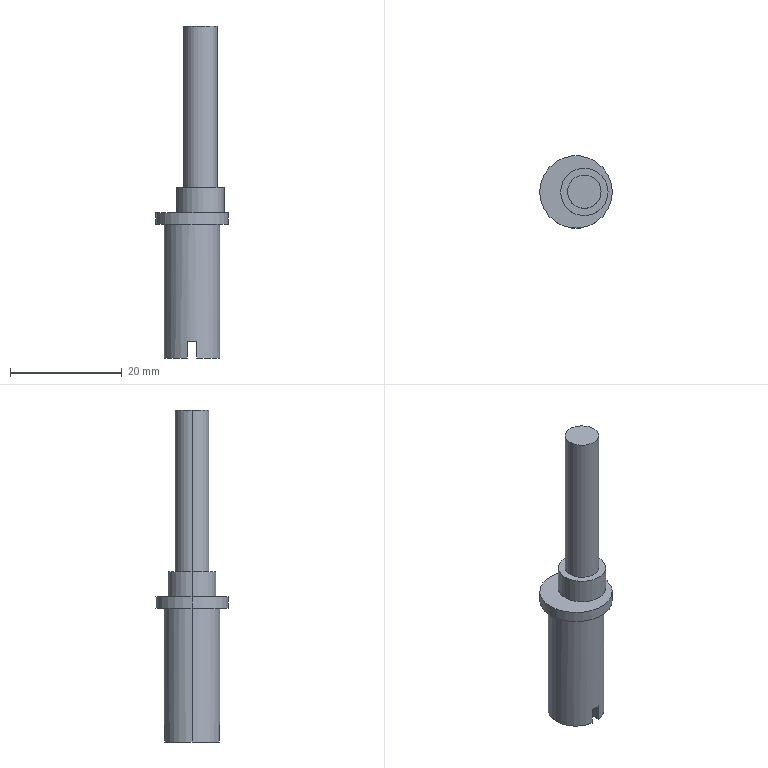Part | SolidWorks | features ICE 5, Extrusion 1 | 1 solid | 17 faces | box 13 x 13 x 59.5 mm | volume 3175 mm3 | plane 9 | cylinder 8 | commonest cylinder face diameters 6 x2 8.5 x2 10 x2 13 x2
STEP:
#1=CARTESIAN_POINT('',(-5.,0.,24.));
#2=VERTEX_POINT('',#1);
#3=CARTESIAN_POINT('',(5.,0.,24.));
#4=VERTEX_POINT('',#3);
#5=CARTESIAN_POINT('',(0.,0.,24.));
#6=DIRECTION('',(0.,0.,-1.));
#7=DIRECTION('',(-1.,0.,0.));
#8=AXIS2_PLACEMENT_3D('',#5,#6,#7);
#9=CIRCLE('',#8,5.);
#10=EDGE_CURVE('',#2,#4,#9,.T.);
#11=ORIENTED_EDGE('',*,*,#10,.T.);
#12=CARTESIAN_POINT('',(5.,0.,0.));
#13=VERTEX_POINT('',#12);
#14=CARTESIAN_POINT('',(5.,0.,25.));
#15=DIRECTION('',(0.,0.,-1.));
#16=VECTOR('',#15,1000.);
#17=LINE('',#14,#16);
#18=EDGE_CURVE('',#4,#13,#17,.T.);
#19=ORIENTED_EDGE('',*,*,#18,.T.);
#20=CARTESIAN_POINT('',(0.85,4.927,0.));
#21=VERTEX_POINT('',#20);
#22=CARTESIAN_POINT('',(0.,0.,0.));
#23=DIRECTION('',(0.,0.,1.));
#24=DIRECTION('',(1.,0.,0.));
#25=AXIS2_PLACEMENT_3D('',#22,#23,#24);
#26=CIRCLE('',#25,5.);
#27=EDGE_CURVE('',#13,#21,#26,.T.);
#28=ORIENTED_EDGE('',*,*,#27,.T.);
#29=CARTESIAN_POINT('',(0.85,4.927,3.));
#30=VERTEX_POINT('',#29);
#31=CARTESIAN_POINT('',(0.85,4.927,25.));
#32=DIRECTION('',(0.,0.,1.));
#33=VECTOR('',#32,1000.);
#34=LINE('',#31,#33);
#35=EDGE_CURVE('',#21,#30,#34,.T.);
#36=ORIENTED_EDGE('',*,*,#35,.T.);
#37=CARTESIAN_POINT('',(-0.85,4.927,3.));
#38=VERTEX_POINT('',#37);
#39=CARTESIAN_POINT('',(0.,0.,3.));
#40=DIRECTION('',(0.,0.,-1.));
#41=DIRECTION('',(-1.,0.,0.));
#42=AXIS2_PLACEMENT_3D('',#39,#40,#41);
#43=CIRCLE('',#42,5.);
#44=EDGE_CURVE('',#38,#30,#43,.T.);
#45=ORIENTED_EDGE('',*,*,#44,.F.);
#46=CARTESIAN_POINT('',(-0.85,4.927,0.));
#47=VERTEX_POINT('',#46);
#48=CARTESIAN_POINT('',(-0.85,4.927,25.));
#49=DIRECTION('',(0.,0.,-1.));
#50=VECTOR('',#49,1000.);
#51=LINE('',#48,#50);
#52=EDGE_CURVE('',#38,#47,#51,.T.);
#53=ORIENTED_EDGE('',*,*,#52,.T.);
#54=CARTESIAN_POINT('',(-5.,0.,0.));
#55=VERTEX_POINT('',#54);
#56=CARTESIAN_POINT('',(0.,0.,0.));
#57=DIRECTION('',(0.,0.,1.));
#58=DIRECTION('',(1.,0.,0.));
#59=AXIS2_PLACEMENT_3D('',#56,#57,#58);
#60=CIRCLE('',#59,5.);
#61=EDGE_CURVE('',#47,#55,#60,.T.);
#62=ORIENTED_EDGE('',*,*,#61,.T.);
#63=CARTESIAN_POINT('',(-5.,0.,25.));
#64=DIRECTION('',(0.,0.,-1.));
#65=VECTOR('',#64,1000.);
#66=LINE('',#63,#65);
#67=EDGE_CURVE('',#2,#55,#66,.T.);
#68=ORIENTED_EDGE('',*,*,#67,.F.);
#69=EDGE_LOOP('',(#11,#19,#28,#36,#45,#53,#62,#68));
#70=FACE_OUTER_BOUND('',#69,.T.);
#71=CARTESIAN_POINT('',(0.,0.,25.));
#72=DIRECTION('',(0.,0.,-1.));
#73=DIRECTION('',(-1.,0.,0.));
#74=AXIS2_PLACEMENT_3D('',#71,#72,#73);
#75=CYLINDRICAL_SURFACE('',#74,5.);
#76=ADVANCED_FACE('',(#70),#75,.T.);
#77=CARTESIAN_POINT('',(4.5,0.,59.5));
#78=VERTEX_POINT('',#77);
#79=CARTESIAN_POINT('',(-1.5,0.,59.5));
#80=VERTEX_POINT('',#79);
#81=CARTESIAN_POINT('',(1.5,0.,59.5));
#82=DIRECTION('',(0.,0.,1.));
#83=DIRECTION('',(1.,0.,0.));
#84=AXIS2_PLACEMENT_3D('',#81,#82,#83);
#85=CIRCLE('',#84,3.);
#86=EDGE_CURVE('',#78,#80,#85,.T.);
#87=ORIENTED_EDGE('',*,*,#86,.F.);
#88=CARTESIAN_POINT('',(4.5,0.,30.5));
#89=VERTEX_POINT('',#88);
#90=CARTESIAN_POINT('',(4.5,0.,59.5));
#91=DIRECTION('',(0.,0.,-1.));
#92=VECTOR('',#91,1000.);
#93=LINE('',#90,#92);
#94=EDGE_CURVE('',#78,#89,#93,.T.);
#95=ORIENTED_EDGE('',*,*,#94,.T.);
#96=CARTESIAN_POINT('',(-1.5,0.,30.5));
#97=VERTEX_POINT('',#96);
#98=CARTESIAN_POINT('',(1.5,0.,30.5));
#99=DIRECTION('',(0.,0.,1.));
#100=DIRECTION('',(1.,0.,0.));
#101=AXIS2_PLACEMENT_3D('',#98,#99,#100);
#102=CIRCLE('',#101,3.);
#103=EDGE_CURVE('',#89,#97,#102,.T.);
#104=ORIENTED_EDGE('',*,*,#103,.T.);
#105=CARTESIAN_POINT('',(-1.5,0.,59.5));
#106=DIRECTION('',(0.,0.,-1.));
#107=VECTOR('',#106,1000.);
#108=LINE('',#105,#107);
#109=EDGE_CURVE('',#80,#97,#108,.T.);
#110=ORIENTED_EDGE('',*,*,#109,.F.);
#111=EDGE_LOOP('',(#87,#95,#104,#110));
#112=FACE_OUTER_BOUND('',#111,.T.);
#113=CARTESIAN_POINT('',(1.5,0.,59.5));
#114=DIRECTION('',(0.,0.,-1.));
#115=DIRECTION('',(-1.,0.,0.));
#116=AXIS2_PLACEMENT_3D('',#113,#114,#115);
#117=CYLINDRICAL_SURFACE('',#116,3.);
#118=ADVANCED_FACE('',(#112),#117,.T.);
#119=CARTESIAN_POINT('',(5.75,0.,30.5));
#120=VERTEX_POINT('',#119);
#121=CARTESIAN_POINT('',(-2.75,0.,30.5));
#122=VERTEX_POINT('',#121);
#123=CARTESIAN_POINT('',(1.5,0.,30.5));
#124=DIRECTION('',(0.,0.,1.));
#125=DIRECTION('',(1.,0.,0.));
#126=AXIS2_PLACEMENT_3D('',#123,#124,#125);
#127=CIRCLE('',#126,4.25);
#128=EDGE_CURVE('',#120,#122,#127,.T.);
#129=ORIENTED_EDGE('',*,*,#128,.F.);
#130=CARTESIAN_POINT('',(5.75,0.,26.));
#131=VERTEX_POINT('',#130);
#132=CARTESIAN_POINT('',(5.75,0.,30.5));
#133=DIRECTION('',(0.,0.,-1.));
#134=VECTOR('',#133,1000.);
#135=LINE('',#132,#134);
#136=EDGE_CURVE('',#120,#131,#135,.T.);
#137=ORIENTED_EDGE('',*,*,#136,.T.);
#138=CARTESIAN_POINT('',(-2.75,0.,26.));
#139=VERTEX_POINT('',#138);
#140=CARTESIAN_POINT('',(1.5,0.,26.));
#141=DIRECTION('',(0.,0.,1.));
#142=DIRECTION('',(1.,0.,0.));
#143=AXIS2_PLACEMENT_3D('',#140,#141,#142);
#144=CIRCLE('',#143,4.25);
#145=EDGE_CURVE('',#131,#139,#144,.T.);
#146=ORIENTED_EDGE('',*,*,#145,.T.);
#147=CARTESIAN_POINT('',(-2.75,0.,30.5));
#148=DIRECTION('',(0.,0.,-1.));
#149=VECTOR('',#148,1000.);
#150=LINE('',#147,#149);
#151=EDGE_CURVE('',#122,#139,#150,.T.);
#152=ORIENTED_EDGE('',*,*,#151,.F.);
#153=EDGE_LOOP('',(#129,#137,#146,#152));
#154=FACE_OUTER_BOUND('',#153,.T.);
#155=CARTESIAN_POINT('',(1.5,0.,30.5));
#156=DIRECTION('',(0.,0.,-1.));
#157=DIRECTION('',(-1.,0.,0.));
#158=AXIS2_PLACEMENT_3D('',#155,#156,#157);
#159=CYLINDRICAL_SURFACE('',#158,4.25);
#160=ADVANCED_FACE('',(#154),#159,.T.);
#161=CARTESIAN_POINT('',(6.5,0.,26.));
#162=VERTEX_POINT('',#161);
#163=CARTESIAN_POINT('',(-6.5,0.,26.));
#164=VERTEX_POINT('',#163);
#165=CARTESIAN_POINT('',(0.,0.,26.));
#166=DIRECTION('',(0.,0.,1.));
#167=DIRECTION('',(1.,0.,0.));
#168=AXIS2_PLACEMENT_3D('',#165,#166,#167);
#169=CIRCLE('',#168,6.5);
#170=EDGE_CURVE('',#162,#164,#169,.T.);
#171=ORIENTED_EDGE('',*,*,#170,.F.);
#172=CARTESIAN_POINT('',(6.5,0.,24.));
#173=VERTEX_POINT('',#172);
#174=CARTESIAN_POINT('',(6.5,0.,26.));
#175=DIRECTION('',(0.,0.,-1.));
#176=VECTOR('',#175,1000.);
#177=LINE('',#174,#176);
#178=EDGE_CURVE('',#162,#173,#177,.T.);
#179=ORIENTED_EDGE('',*,*,#178,.T.);
#180=CARTESIAN_POINT('',(-6.5,0.,24.));
#181=VERTEX_POINT('',#180);
#182=CARTESIAN_POINT('',(0.,0.,24.));
#183=DIRECTION('',(0.,0.,-1.));
#184=DIRECTION('',(-1.,0.,0.));
#185=AXIS2_PLACEMENT_3D('',#182,#183,#184);
#186=CIRCLE('',#185,6.5);
#187=EDGE_CURVE('',#181,#173,#186,.T.);
#188=ORIENTED_EDGE('',*,*,#187,.F.);
#189=CARTESIAN_POINT('',(-6.5,0.,26.));
#190=DIRECTION('',(0.,0.,-1.));
#191=VECTOR('',#190,1000.);
#192=LINE('',#189,#191);
#193=EDGE_CURVE('',#164,#181,#192,.T.);
#194=ORIENTED_EDGE('',*,*,#193,.F.);
#195=EDGE_LOOP('',(#171,#179,#188,#194));
#196=FACE_OUTER_BOUND('',#195,.T.);
#197=CARTESIAN_POINT('',(0.,0.,26.));
#198=DIRECTION('',(0.,0.,-1.));
#199=DIRECTION('',(-1.,0.,0.));
#200=AXIS2_PLACEMENT_3D('',#197,#198,#199);
#201=CYLINDRICAL_SURFACE('',#200,6.5);
#202=ADVANCED_FACE('',(#196),#201,.T.);
#203=ORIENTED_EDGE('',*,*,#178,.F.);
#204=CARTESIAN_POINT('',(0.,0.,26.));
#205=DIRECTION('',(0.,0.,1.));
#206=DIRECTION('',(1.,0.,0.));
#207=AXIS2_PLACEMENT_3D('',#204,#205,#206);
#208=CIRCLE('',#207,6.5);
#209=EDGE_CURVE('',#164,#162,#208,.T.);
#210=ORIENTED_EDGE('',*,*,#209,.F.);
#211=ORIENTED_EDGE('',*,*,#193,.T.);
#212=CARTESIAN_POINT('',(0.,0.,24.));
#213=DIRECTION('',(0.,0.,-1.));
#214=DIRECTION('',(-1.,0.,0.));
#215=AXIS2_PLACEMENT_3D('',#212,#213,#214);
#216=CIRCLE('',#215,6.5);
#217=EDGE_CURVE('',#173,#181,#216,.T.);
#218=ORIENTED_EDGE('',*,*,#217,.F.);
#219=EDGE_LOOP('',(#203,#210,#211,#218));
#220=FACE_OUTER_BOUND('',#219,.T.);
#221=CARTESIAN_POINT('',(0.,0.,26.));
#222=DIRECTION('',(0.,0.,-1.));
#223=DIRECTION('',(-1.,0.,0.));
#224=AXIS2_PLACEMENT_3D('',#221,#222,#223);
#225=CYLINDRICAL_SURFACE('',#224,6.5);
#226=ADVANCED_FACE('',(#220),#225,.T.);
#227=CARTESIAN_POINT('',(1.5,0.,26.));
#228=DIRECTION('',(0.,0.,1.));
#229=DIRECTION('',(1.,0.,0.));
#230=AXIS2_PLACEMENT_3D('',#227,#228,#229);
#231=CIRCLE('',#230,4.25);
#232=EDGE_CURVE('',#139,#131,#231,.T.);
#233=ORIENTED_EDGE('',*,*,#232,.F.);
#234=ORIENTED_EDGE('',*,*,#145,.F.);
#235=EDGE_LOOP('',(#233,#234));
#236=FACE_BOUND('',#235,.T.);
#237=ORIENTED_EDGE('',*,*,#209,.T.);
#238=ORIENTED_EDGE('',*,*,#170,.T.);
#239=EDGE_LOOP('',(#237,#238));
#240=FACE_OUTER_BOUND('',#239,.T.);
#241=CARTESIAN_POINT('',(0.,0.,26.));
#242=DIRECTION('',(0.,0.,1.));
#243=DIRECTION('',(1.,0.,0.));
#244=AXIS2_PLACEMENT_3D('',#241,#242,#243);
#245=PLANE('',#244);
#246=ADVANCED_FACE('',(#236,#240),#245,.T.);
#247=ORIENTED_EDGE('',*,*,#136,.F.);
#248=CARTESIAN_POINT('',(1.5,0.,30.5));
#249=DIRECTION('',(0.,0.,1.));
#250=DIRECTION('',(1.,0.,0.));
#251=AXIS2_PLACEMENT_3D('',#248,#249,#250);
#252=CIRCLE('',#251,4.25);
#253=EDGE_CURVE('',#122,#120,#252,.T.);
#254=ORIENTED_EDGE('',*,*,#253,.F.);
#255=ORIENTED_EDGE('',*,*,#151,.T.);
#256=ORIENTED_EDGE('',*,*,#232,.T.);
#257=EDGE_LOOP('',(#247,#254,#255,#256));
#258=FACE_OUTER_BOUND('',#257,.T.);
#259=CARTESIAN_POINT('',(1.5,0.,30.5));
#260=DIRECTION('',(0.,0.,-1.));
#261=DIRECTION('',(-1.,0.,0.));
#262=AXIS2_PLACEMENT_3D('',#259,#260,#261);
#263=CYLINDRICAL_SURFACE('',#262,4.25);
#264=ADVANCED_FACE('',(#258),#263,.T.);
#265=CARTESIAN_POINT('',(1.5,0.,30.5));
#266=DIRECTION('',(0.,0.,1.));
#267=DIRECTION('',(1.,0.,0.));
#268=AXIS2_PLACEMENT_3D('',#265,#266,#267);
#269=CIRCLE('',#268,3.);
#270=EDGE_CURVE('',#97,#89,#269,.T.);
#271=ORIENTED_EDGE('',*,*,#270,.F.);
#272=ORIENTED_EDGE('',*,*,#103,.F.);
#273=EDGE_LOOP('',(#271,#272));
#274=FACE_BOUND('',#273,.T.);
#275=ORIENTED_EDGE('',*,*,#253,.T.);
#276=ORIENTED_EDGE('',*,*,#128,.T.);
#277=EDGE_LOOP('',(#275,#276));
#278=FACE_OUTER_BOUND('',#277,.T.);
#279=CARTESIAN_POINT('',(1.5,0.,30.5));
#280=DIRECTION('',(0.,0.,1.));
#281=DIRECTION('',(1.,0.,0.));
#282=AXIS2_PLACEMENT_3D('',#279,#280,#281);
#283=PLANE('',#282);
#284=ADVANCED_FACE('',(#274,#278),#283,.T.);
#285=ORIENTED_EDGE('',*,*,#94,.F.);
#286=CARTESIAN_POINT('',(1.5,0.,59.5));
#287=DIRECTION('',(0.,0.,1.));
#288=DIRECTION('',(1.,0.,0.));
#289=AXIS2_PLACEMENT_3D('',#286,#287,#288);
#290=CIRCLE('',#289,3.);
#291=EDGE_CURVE('',#80,#78,#290,.T.);
#292=ORIENTED_EDGE('',*,*,#291,.F.);
#293=ORIENTED_EDGE('',*,*,#109,.T.);
#294=ORIENTED_EDGE('',*,*,#270,.T.);
#295=EDGE_LOOP('',(#285,#292,#293,#294));
#296=FACE_OUTER_BOUND('',#295,.T.);
#297=CARTESIAN_POINT('',(1.5,0.,59.5));
#298=DIRECTION('',(0.,0.,-1.));
#299=DIRECTION('',(-1.,0.,0.));
#300=AXIS2_PLACEMENT_3D('',#297,#298,#299);
#301=CYLINDRICAL_SURFACE('',#300,3.);
#302=ADVANCED_FACE('',(#296),#301,.T.);
#303=ORIENTED_EDGE('',*,*,#291,.T.);
#304=ORIENTED_EDGE('',*,*,#86,.T.);
#305=EDGE_LOOP('',(#303,#304));
#306=FACE_OUTER_BOUND('',#305,.T.);
#307=CARTESIAN_POINT('',(1.5,0.,59.5));
#308=DIRECTION('',(0.,0.,1.));
#309=DIRECTION('',(1.,0.,0.));
#310=AXIS2_PLACEMENT_3D('',#307,#308,#309);
#311=PLANE('',#310);
#312=ADVANCED_FACE('',(#306),#311,.T.);
#313=ORIENTED_EDGE('',*,*,#10,.F.);
#314=CARTESIAN_POINT('',(0.,0.,24.));
#315=DIRECTION('',(0.,0.,-1.));
#316=DIRECTION('',(-1.,0.,0.));
#317=AXIS2_PLACEMENT_3D('',#314,#315,#316);
#318=CIRCLE('',#317,5.);
#319=EDGE_CURVE('',#4,#2,#318,.T.);
#320=ORIENTED_EDGE('',*,*,#319,.F.);
#321=EDGE_LOOP('',(#313,#320));
#322=FACE_BOUND('',#321,.T.);
#323=ORIENTED_EDGE('',*,*,#187,.T.);
#324=ORIENTED_EDGE('',*,*,#217,.T.);
#325=EDGE_LOOP('',(#323,#324));
#326=FACE_OUTER_BOUND('',#325,.T.);
#327=CARTESIAN_POINT('',(0.,0.,24.));
#328=DIRECTION('',(0.,0.,-1.));
#329=DIRECTION('',(-1.,0.,0.));
#330=AXIS2_PLACEMENT_3D('',#327,#328,#329);
#331=PLANE('',#330);
#332=ADVANCED_FACE('',(#322,#326),#331,.T.);
#333=CARTESIAN_POINT('',(0.85,-4.927,0.));
#334=VERTEX_POINT('',#333);
#335=CARTESIAN_POINT('',(0.,0.,0.));
#336=DIRECTION('',(0.,0.,1.));
#337=DIRECTION('',(1.,0.,0.));
#338=AXIS2_PLACEMENT_3D('',#335,#336,#337);
#339=CIRCLE('',#338,5.);
#340=EDGE_CURVE('',#334,#13,#339,.T.);
#341=ORIENTED_EDGE('',*,*,#340,.F.);
#342=CARTESIAN_POINT('',(0.85,0.,0.));
#343=DIRECTION('',(0.,1.,0.));
#344=VECTOR('',#343,1000.);
#345=LINE('',#342,#344);
#346=EDGE_CURVE('',#334,#21,#345,.T.);
#347=ORIENTED_EDGE('',*,*,#346,.T.);
#348=ORIENTED_EDGE('',*,*,#27,.F.);
#349=EDGE_LOOP('',(#341,#347,#348));
#350=FACE_OUTER_BOUND('',#349,.T.);
#351=CARTESIAN_POINT('',(0.,0.,0.));
#352=DIRECTION('',(0.,0.,1.));
#353=DIRECTION('',(1.,0.,0.));
#354=AXIS2_PLACEMENT_3D('',#351,#352,#353);
#355=PLANE('',#354);
#356=ADVANCED_FACE('',(#350),#355,.F.);
#357=CARTESIAN_POINT('',(0.85,-4.927,3.));
#358=VERTEX_POINT('',#357);
#359=CARTESIAN_POINT('',(0.85,5.966,3.));
#360=DIRECTION('',(0.,-1.,0.));
#361=VECTOR('',#360,1000.);
#362=LINE('',#359,#361);
#363=EDGE_CURVE('',#30,#358,#362,.T.);
#364=ORIENTED_EDGE('',*,*,#363,.F.);
#365=ORIENTED_EDGE('',*,*,#35,.F.);
#366=ORIENTED_EDGE('',*,*,#346,.F.);
#367=CARTESIAN_POINT('',(0.85,-4.927,25.));
#368=DIRECTION('',(0.,0.,-1.));
#369=VECTOR('',#368,1000.);
#370=LINE('',#367,#369);
#371=EDGE_CURVE('',#358,#334,#370,.T.);
#372=ORIENTED_EDGE('',*,*,#371,.F.);
#373=EDGE_LOOP('',(#364,#365,#366,#372));
#374=FACE_OUTER_BOUND('',#373,.T.);
#375=CARTESIAN_POINT('',(0.85,5.966,3.));
#376=DIRECTION('',(1.,0.,0.));
#377=DIRECTION('',(0.,0.,-1.));
#378=AXIS2_PLACEMENT_3D('',#375,#376,#377);
#379=PLANE('',#378);
#380=ADVANCED_FACE('',(#374),#379,.F.);
#381=ORIENTED_EDGE('',*,*,#61,.F.);
#382=CARTESIAN_POINT('',(-0.85,-4.927,0.));
#383=VERTEX_POINT('',#382);
#384=CARTESIAN_POINT('',(-0.85,0.,0.));
#385=DIRECTION('',(0.,-1.,0.));
#386=VECTOR('',#385,1000.);
#387=LINE('',#384,#386);
#388=EDGE_CURVE('',#47,#383,#387,.T.);
#389=ORIENTED_EDGE('',*,*,#388,.T.);
#390=CARTESIAN_POINT('',(0.,0.,0.));
#391=DIRECTION('',(0.,0.,1.));
#392=DIRECTION('',(1.,0.,0.));
#393=AXIS2_PLACEMENT_3D('',#390,#391,#392);
#394=CIRCLE('',#393,5.);
#395=EDGE_CURVE('',#55,#383,#394,.T.);
#396=ORIENTED_EDGE('',*,*,#395,.F.);
#397=EDGE_LOOP('',(#381,#389,#396));
#398=FACE_OUTER_BOUND('',#397,.T.);
#399=CARTESIAN_POINT('',(0.,0.,0.));
#400=DIRECTION('',(0.,0.,1.));
#401=DIRECTION('',(1.,0.,0.));
#402=AXIS2_PLACEMENT_3D('',#399,#400,#401);
#403=PLANE('',#402);
#404=ADVANCED_FACE('',(#398),#403,.F.);
#405=CARTESIAN_POINT('',(-0.85,-4.927,3.));
#406=VERTEX_POINT('',#405);
#407=CARTESIAN_POINT('',(-0.85,5.966,3.));
#408=DIRECTION('',(0.,1.,0.));
#409=VECTOR('',#408,1000.);
#410=LINE('',#407,#409);
#411=EDGE_CURVE('',#406,#38,#410,.T.);
#412=ORIENTED_EDGE('',*,*,#411,.F.);
#413=CARTESIAN_POINT('',(-0.85,-4.927,25.));
#414=DIRECTION('',(0.,0.,1.));
#415=VECTOR('',#414,1000.);
#416=LINE('',#413,#415);
#417=EDGE_CURVE('',#383,#406,#416,.T.);
#418=ORIENTED_EDGE('',*,*,#417,.F.);
#419=ORIENTED_EDGE('',*,*,#388,.F.);
#420=ORIENTED_EDGE('',*,*,#52,.F.);
#421=EDGE_LOOP('',(#412,#418,#419,#420));
#422=FACE_OUTER_BOUND('',#421,.T.);
#423=CARTESIAN_POINT('',(-0.85,5.966,3.));
#424=DIRECTION('',(-1.,0.,0.));
#425=DIRECTION('',(0.,0.,1.));
#426=AXIS2_PLACEMENT_3D('',#423,#424,#425);
#427=PLANE('',#426);
#428=ADVANCED_FACE('',(#422),#427,.F.);
#429=ORIENTED_EDGE('',*,*,#44,.T.);
#430=ORIENTED_EDGE('',*,*,#363,.T.);
#431=CARTESIAN_POINT('',(0.,0.,3.));
#432=DIRECTION('',(0.,0.,-1.));
#433=DIRECTION('',(-1.,0.,0.));
#434=AXIS2_PLACEMENT_3D('',#431,#432,#433);
#435=CIRCLE('',#434,5.);
#436=EDGE_CURVE('',#358,#406,#435,.T.);
#437=ORIENTED_EDGE('',*,*,#436,.T.);
#438=ORIENTED_EDGE('',*,*,#411,.T.);
#439=EDGE_LOOP('',(#429,#430,#437,#438));
#440=FACE_OUTER_BOUND('',#439,.T.);
#441=CARTESIAN_POINT('',(0.,0.,3.));
#442=DIRECTION('',(0.,0.,-1.));
#443=DIRECTION('',(-1.,0.,0.));
#444=AXIS2_PLACEMENT_3D('',#441,#442,#443);
#445=PLANE('',#444);
#446=ADVANCED_FACE('',(#440),#445,.T.);
#447=ORIENTED_EDGE('',*,*,#18,.F.);
#448=ORIENTED_EDGE('',*,*,#319,.T.);
#449=ORIENTED_EDGE('',*,*,#67,.T.);
#450=ORIENTED_EDGE('',*,*,#395,.T.);
#451=ORIENTED_EDGE('',*,*,#417,.T.);
#452=ORIENTED_EDGE('',*,*,#436,.F.);
#453=ORIENTED_EDGE('',*,*,#371,.T.);
#454=ORIENTED_EDGE('',*,*,#340,.T.);
#455=EDGE_LOOP('',(#447,#448,#449,#450,#451,#452,#453,#454));
#456=FACE_OUTER_BOUND('',#455,.T.);
#457=CARTESIAN_POINT('',(0.,0.,25.));
#458=DIRECTION('',(0.,0.,-1.));
#459=DIRECTION('',(-1.,0.,0.));
#460=AXIS2_PLACEMENT_3D('',#457,#458,#459);
#461=CYLINDRICAL_SURFACE('',#460,5.);
#462=ADVANCED_FACE('',(#456),#461,.T.);
#463=CLOSED_SHELL('',(#76,#118,#160,#202,#226,#246,#264,#284,#302,#312,#332,#356,#380,#404,#428,#446,#462));
#464=MANIFOLD_SOLID_BREP('',#463);
#465=CARTESIAN_POINT('',(0.,0.,0.));
#466=DIRECTION('',(0.,0.,1.));
#467=DIRECTION('',(1.,0.,0.));
#468=AXIS2_PLACEMENT_3D('',#465,#466,#467);
#469=(LENGTH_UNIT()NAMED_UNIT(*)SI_UNIT(.MILLI.,.METRE.));
#470=UNCERTAINTY_MEASURE_WITH_UNIT(LENGTH_MEASURE(0.00001),#469,'','');
#471=(NAMED_UNIT(*)PLANE_ANGLE_UNIT()SI_UNIT($,.RADIAN.));
#472=(NAMED_UNIT(*)SI_UNIT($,.STERADIAN.)SOLID_ANGLE_UNIT());
#473=(GEOMETRIC_REPRESENTATION_CONTEXT(3)GLOBAL_UNCERTAINTY_ASSIGNED_CONTEXT((#470))GLOBAL_UNIT_ASSIGNED_CONTEXT((#469,#471,#472))REPRESENTATION_CONTEXT('',''));
#474=ADVANCED_BREP_SHAPE_REPRESENTATION('',(#464,#468),#473);